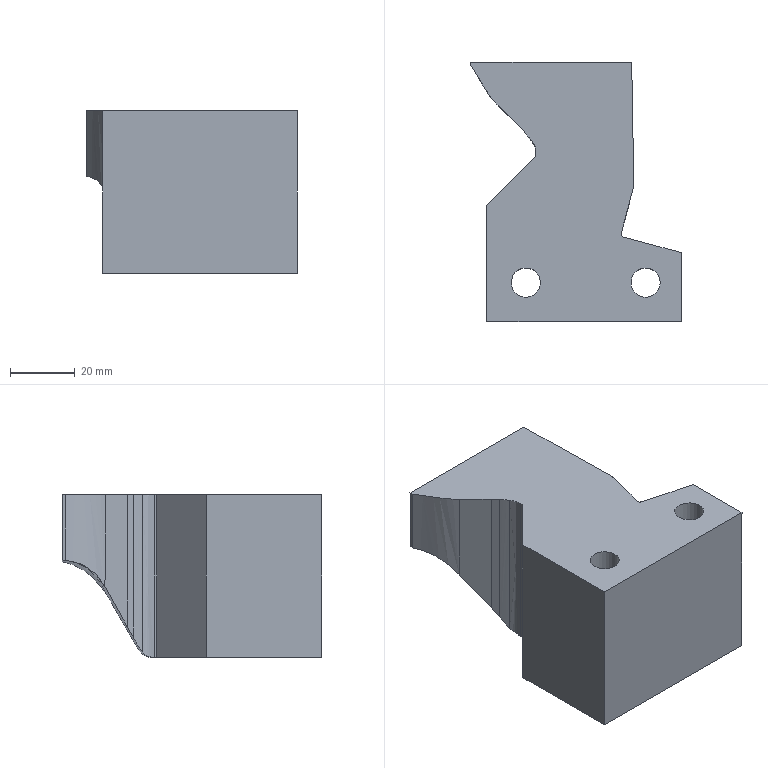Part | NX | features solid 2 | 1 solid | 34 faces | box 65 x 80 x 50.25 mm | volume 149618 mm3 | plane 17 | cylinder 11 | spline 5 | cone 1 | commonest cylinder face diameters 9.009 x2 10 x2 14.507 x2 2 x1 6.805 x1 7 x1